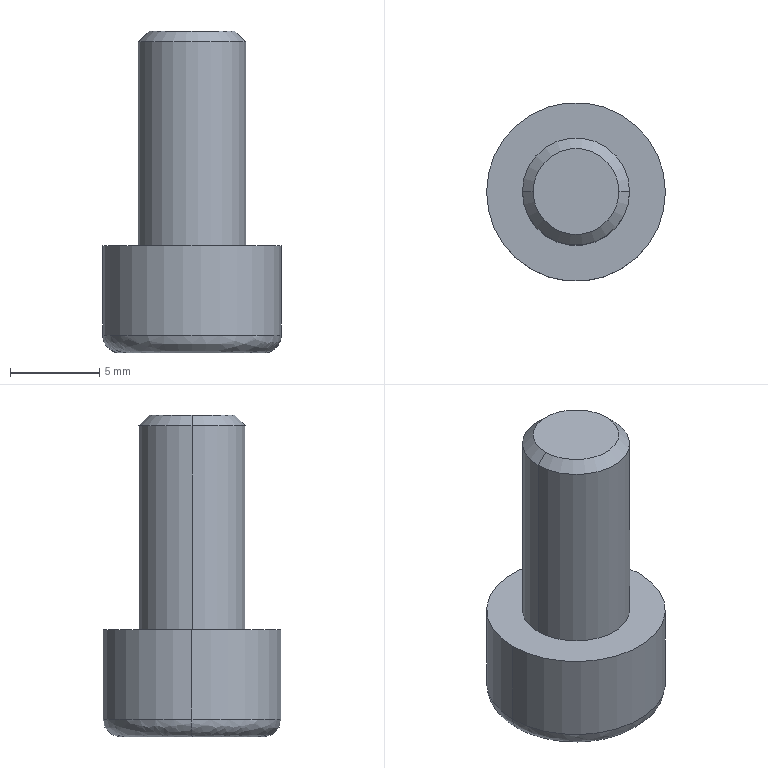Part | STEP file | LE-YZS-M6X12_PN_0002 | 1 solid | 25 faces | box 10 x 10 x 18 mm | volume 726.537 mm3 | plane 15 | cylinder 4 | cone 4 | spline 2 | commonest cylinder face diameters 6 x2 10 x2
STEP:
#1=CARTESIAN_POINT('',(-5.,0.,-5.));
#2=VERTEX_POINT('',#1);
#3=CARTESIAN_POINT('',(5.,0.,-5.));
#4=VERTEX_POINT('',#3);
#5=CARTESIAN_POINT('',(0.,0.,-5.));
#6=DIRECTION('',(0.,0.,1.));
#7=DIRECTION('',(1.,0.,0.));
#8=AXIS2_PLACEMENT_3D('',#5,#6,#7);
#9=CIRCLE('',#8,5.);
#10=EDGE_CURVE('',#2,#4,#9,.T.);
#11=ORIENTED_EDGE('',*,*,#10,.F.);
#12=CARTESIAN_POINT('',(-4.,0.,-6.));
#13=VERTEX_POINT('',#12);
#14=CARTESIAN_POINT('',(-4.,0.,-5.));
#15=DIRECTION('',(0.,-1.,0.));
#16=DIRECTION('',(-1.,0.,0.));
#17=AXIS2_PLACEMENT_3D('',#14,#15,#16);
#18=CIRCLE('',#17,1.);
#19=EDGE_CURVE('',#2,#13,#18,.T.);
#20=ORIENTED_EDGE('',*,*,#19,.T.);
#21=CARTESIAN_POINT('',(4.,0.,-6.));
#22=VERTEX_POINT('',#21);
#23=CARTESIAN_POINT('',(-4.,0.,-6.));
#24=CARTESIAN_POINT('',(-4.,-8.,-6.));
#25=CARTESIAN_POINT('',(4.,-8.,-6.));
#26=CARTESIAN_POINT('',(4.,0.,-6.));
#27=(BOUNDED_CURVE()B_SPLINE_CURVE(3,(#23,#24,#25,#26),.UNSPECIFIED.,.F.,.F.)B_SPLINE_CURVE_WITH_KNOTS((4,4),(0.,1.),.UNSPECIFIED.)CURVE()GEOMETRIC_REPRESENTATION_ITEM()RATIONAL_B_SPLINE_CURVE((1.,0.3333,0.3333,1.))REPRESENTATION_ITEM(''));
#28=EDGE_CURVE('',#13,#22,#27,.T.);
#29=ORIENTED_EDGE('',*,*,#28,.T.);
#30=CARTESIAN_POINT('',(4.,0.,-5.));
#31=DIRECTION('',(0.,1.,0.));
#32=DIRECTION('',(1.,0.,0.));
#33=AXIS2_PLACEMENT_3D('',#30,#31,#32);
#34=CIRCLE('',#33,1.);
#35=EDGE_CURVE('',#4,#22,#34,.T.);
#36=ORIENTED_EDGE('',*,*,#35,.F.);
#37=EDGE_LOOP('',(#11,#20,#29,#36));
#38=FACE_OUTER_BOUND('',#37,.T.);
#39=CARTESIAN_POINT('',(-5.,0.,-5.));
#40=CARTESIAN_POINT('',(-5.,-10.,-5.));
#41=CARTESIAN_POINT('',(5.,-10.,-5.));
#42=CARTESIAN_POINT('',(5.,0.,-5.));
#43=CARTESIAN_POINT('',(-5.,0.,-5.586));
#44=CARTESIAN_POINT('',(-5.,-10.,-5.586));
#45=CARTESIAN_POINT('',(5.,-10.,-5.586));
#46=CARTESIAN_POINT('',(5.,0.,-5.586));
#47=CARTESIAN_POINT('',(-4.586,0.,-6.));
#48=CARTESIAN_POINT('',(-4.586,-9.172,-6.));
#49=CARTESIAN_POINT('',(4.586,-9.172,-6.));
#50=CARTESIAN_POINT('',(4.586,0.,-6.));
#51=CARTESIAN_POINT('',(-4.,0.,-6.));
#52=CARTESIAN_POINT('',(-4.,-8.,-6.));
#53=CARTESIAN_POINT('',(4.,-8.,-6.));
#54=CARTESIAN_POINT('',(4.,0.,-6.));
#55=(BOUNDED_SURFACE()B_SPLINE_SURFACE(3,3,((#39,#40,#41,#42),(#43,#44,#45,#46),(#47,#48,#49,#50),(#51,#52,#53,#54)),.UNSPECIFIED.,.F.,.F.,.F.)B_SPLINE_SURFACE_WITH_KNOTS((4,4),(4,4),(0.,1.),(0.,1.),.UNSPECIFIED.)GEOMETRIC_REPRESENTATION_ITEM()RATIONAL_B_SPLINE_SURFACE(((1.,0.3333,0.3333,1.),(0.8047,0.2682,0.2682,0.8047),(0.8047,0.2682,0.2682,0.8047),(1.,0.3333,0.3333,1.)))REPRESENTATION_ITEM('')SURFACE());
#56=ADVANCED_FACE('',(#38),#55,.T.);
#57=CARTESIAN_POINT('',(-3.,0.,11.4));
#58=VERTEX_POINT('',#57);
#59=CARTESIAN_POINT('',(3.,0.,11.4));
#60=VERTEX_POINT('',#59);
#61=CARTESIAN_POINT('',(0.,0.,11.4));
#62=DIRECTION('',(0.,0.,-1.));
#63=DIRECTION('',(-1.,0.,0.));
#64=AXIS2_PLACEMENT_3D('',#61,#62,#63);
#65=CIRCLE('',#64,3.);
#66=EDGE_CURVE('',#58,#60,#65,.T.);
#67=ORIENTED_EDGE('',*,*,#66,.T.);
#68=CARTESIAN_POINT('',(3.,0.,0.));
#69=VERTEX_POINT('',#68);
#70=CARTESIAN_POINT('',(3.,0.,12.));
#71=DIRECTION('',(0.,0.,-1.));
#72=VECTOR('',#71,1000.);
#73=LINE('',#70,#72);
#74=EDGE_CURVE('',#60,#69,#73,.T.);
#75=ORIENTED_EDGE('',*,*,#74,.T.);
#76=CARTESIAN_POINT('',(-3.,0.,0.));
#77=VERTEX_POINT('',#76);
#78=CARTESIAN_POINT('',(0.,0.,0.));
#79=DIRECTION('',(0.,0.,1.));
#80=DIRECTION('',(-1.,0.,0.));
#81=AXIS2_PLACEMENT_3D('',#78,#79,#80);
#82=CIRCLE('',#81,3.);
#83=EDGE_CURVE('',#69,#77,#82,.T.);
#84=ORIENTED_EDGE('',*,*,#83,.T.);
#85=CARTESIAN_POINT('',(-3.,0.,12.));
#86=DIRECTION('',(0.,0.,-1.));
#87=VECTOR('',#86,1000.);
#88=LINE('',#85,#87);
#89=EDGE_CURVE('',#58,#77,#88,.T.);
#90=ORIENTED_EDGE('',*,*,#89,.F.);
#91=EDGE_LOOP('',(#67,#75,#84,#90));
#92=FACE_OUTER_BOUND('',#91,.T.);
#93=CARTESIAN_POINT('',(0.,0.,12.));
#94=DIRECTION('',(0.,0.,-1.));
#95=DIRECTION('',(-1.,0.,0.));
#96=AXIS2_PLACEMENT_3D('',#93,#94,#95);
#97=CYLINDRICAL_SURFACE('',#96,3.);
#98=ADVANCED_FACE('',(#92),#97,.T.);
#99=CARTESIAN_POINT('',(-2.4,0.,12.));
#100=VERTEX_POINT('',#99);
#101=CARTESIAN_POINT('',(2.4,0.,12.));
#102=VERTEX_POINT('',#101);
#103=CARTESIAN_POINT('',(0.,0.,12.));
#104=DIRECTION('',(0.,0.,-1.));
#105=DIRECTION('',(-1.,0.,0.));
#106=AXIS2_PLACEMENT_3D('',#103,#104,#105);
#107=CIRCLE('',#106,2.4);
#108=EDGE_CURVE('',#100,#102,#107,.T.);
#109=ORIENTED_EDGE('',*,*,#108,.T.);
#110=CARTESIAN_POINT('',(3.,0.,11.4));
#111=DIRECTION('',(0.7071,0.,-0.7071));
#112=VECTOR('',#111,1000.);
#113=LINE('',#110,#112);
#114=EDGE_CURVE('',#102,#60,#113,.T.);
#115=ORIENTED_EDGE('',*,*,#114,.T.);
#116=ORIENTED_EDGE('',*,*,#66,.F.);
#117=CARTESIAN_POINT('',(-3.,0.,11.4));
#118=DIRECTION('',(-0.7071,0.,-0.7071));
#119=VECTOR('',#118,1000.);
#120=LINE('',#117,#119);
#121=EDGE_CURVE('',#100,#58,#120,.T.);
#122=ORIENTED_EDGE('',*,*,#121,.F.);
#123=EDGE_LOOP('',(#109,#115,#116,#122));
#124=FACE_OUTER_BOUND('',#123,.T.);
#125=CARTESIAN_POINT('',(0.,0.,11.4));
#126=DIRECTION('',(0.,0.,-1.));
#127=DIRECTION('',(-1.,0.,0.));
#128=AXIS2_PLACEMENT_3D('',#125,#126,#127);
#129=CONICAL_SURFACE('',#128,3.,0.7854);
#130=ADVANCED_FACE('',(#124),#129,.T.);
#131=CARTESIAN_POINT('',(0.,0.,-5.));
#132=DIRECTION('',(0.,0.,1.));
#133=DIRECTION('',(1.,0.,0.));
#134=AXIS2_PLACEMENT_3D('',#131,#132,#133);
#135=CIRCLE('',#134,5.);
#136=EDGE_CURVE('',#4,#2,#135,.T.);
#137=ORIENTED_EDGE('',*,*,#136,.T.);
#138=CARTESIAN_POINT('',(-5.,0.,0.));
#139=VERTEX_POINT('',#138);
#140=CARTESIAN_POINT('',(-5.,0.,-6.));
#141=DIRECTION('',(0.,0.,1.));
#142=VECTOR('',#141,1000.);
#143=LINE('',#140,#142);
#144=EDGE_CURVE('',#2,#139,#143,.T.);
#145=ORIENTED_EDGE('',*,*,#144,.T.);
#146=CARTESIAN_POINT('',(5.,0.,0.));
#147=VERTEX_POINT('',#146);
#148=CARTESIAN_POINT('',(0.,0.,0.));
#149=DIRECTION('',(0.,0.,1.));
#150=DIRECTION('',(1.,0.,0.));
#151=AXIS2_PLACEMENT_3D('',#148,#149,#150);
#152=CIRCLE('',#151,5.);
#153=EDGE_CURVE('',#147,#139,#152,.T.);
#154=ORIENTED_EDGE('',*,*,#153,.F.);
#155=CARTESIAN_POINT('',(5.,0.,-6.));
#156=DIRECTION('',(0.,0.,1.));
#157=VECTOR('',#156,1000.);
#158=LINE('',#155,#157);
#159=EDGE_CURVE('',#4,#147,#158,.T.);
#160=ORIENTED_EDGE('',*,*,#159,.F.);
#161=EDGE_LOOP('',(#137,#145,#154,#160));
#162=FACE_OUTER_BOUND('',#161,.T.);
#163=CARTESIAN_POINT('',(0.,0.,-6.));
#164=DIRECTION('',(0.,0.,1.));
#165=DIRECTION('',(1.,0.,0.));
#166=AXIS2_PLACEMENT_3D('',#163,#164,#165);
#167=CYLINDRICAL_SURFACE('',#166,5.);
#168=ADVANCED_FACE('',(#162),#167,.T.);
#169=CARTESIAN_POINT('',(0.,0.,-1.557));
#170=VERTEX_POINT('',#169);
#171=CARTESIAN_POINT('',(-2.5,0.,-3.));
#172=VERTEX_POINT('',#171);
#173=CARTESIAN_POINT('',(-2.5,0.,-3.));
#174=DIRECTION('',(-0.866,0.,-0.5));
#175=VECTOR('',#174,1000.);
#176=LINE('',#173,#175);
#177=EDGE_CURVE('',#170,#172,#176,.T.);
#178=ORIENTED_EDGE('',*,*,#177,.F.);
#179=CARTESIAN_POINT('',(2.5,0.,-3.));
#180=VERTEX_POINT('',#179);
#181=CARTESIAN_POINT('',(2.5,0.,-3.));
#182=DIRECTION('',(0.866,0.,-0.5));
#183=VECTOR('',#182,1000.);
#184=LINE('',#181,#183);
#185=EDGE_CURVE('',#170,#180,#184,.T.);
#186=ORIENTED_EDGE('',*,*,#185,.T.);
#187=CARTESIAN_POINT('',(2.165,-1.25,-3.));
#188=VERTEX_POINT('',#187);
#189=CARTESIAN_POINT('',(0.,0.,-3.));
#190=DIRECTION('',(0.,0.,1.));
#191=DIRECTION('',(-1.,0.,0.));
#192=AXIS2_PLACEMENT_3D('',#189,#190,#191);
#193=CIRCLE('',#192,2.5);
#194=EDGE_CURVE('',#188,#180,#193,.T.);
#195=ORIENTED_EDGE('',*,*,#194,.F.);
#196=CARTESIAN_POINT('',(0.,-2.5,-3.));
#197=VERTEX_POINT('',#196);
#198=CARTESIAN_POINT('',(0.,0.,-3.));
#199=DIRECTION('',(0.,0.,-1.));
#200=DIRECTION('',(-1.,0.,0.));
#201=AXIS2_PLACEMENT_3D('',#198,#199,#200);
#202=CIRCLE('',#201,2.5);
#203=EDGE_CURVE('',#188,#197,#202,.T.);
#204=ORIENTED_EDGE('',*,*,#203,.T.);
#205=CARTESIAN_POINT('',(-2.165,-1.25,-3.));
#206=VERTEX_POINT('',#205);
#207=CARTESIAN_POINT('',(0.,0.,-3.));
#208=DIRECTION('',(0.,0.,1.));
#209=DIRECTION('',(-1.,0.,0.));
#210=AXIS2_PLACEMENT_3D('',#207,#208,#209);
#211=CIRCLE('',#210,2.5);
#212=EDGE_CURVE('',#206,#197,#211,.T.);
#213=ORIENTED_EDGE('',*,*,#212,.F.);
#214=CARTESIAN_POINT('',(0.,0.,-3.));
#215=DIRECTION('',(0.,0.,1.));
#216=DIRECTION('',(-1.,0.,0.));
#217=AXIS2_PLACEMENT_3D('',#214,#215,#216);
#218=CIRCLE('',#217,2.5);
#219=EDGE_CURVE('',#172,#206,#218,.T.);
#220=ORIENTED_EDGE('',*,*,#219,.F.);
#221=EDGE_LOOP('',(#178,#186,#195,#204,#213,#220));
#222=FACE_OUTER_BOUND('',#221,.T.);
#223=CARTESIAN_POINT('',(0.,0.,-3.));
#224=DIRECTION('',(0.,0.,-1.));
#225=DIRECTION('',(-1.,0.,0.));
#226=AXIS2_PLACEMENT_3D('',#223,#224,#225);
#227=CONICAL_SURFACE('',#226,2.5,1.047);
#228=ADVANCED_FACE('',(#222),#227,.F.);
#229=ORIENTED_EDGE('',*,*,#74,.F.);
#230=CARTESIAN_POINT('',(0.,0.,11.4));
#231=DIRECTION('',(0.,0.,-1.));
#232=DIRECTION('',(-1.,0.,0.));
#233=AXIS2_PLACEMENT_3D('',#230,#231,#232);
#234=CIRCLE('',#233,3.);
#235=EDGE_CURVE('',#60,#58,#234,.T.);
#236=ORIENTED_EDGE('',*,*,#235,.T.);
#237=ORIENTED_EDGE('',*,*,#89,.T.);
#238=CARTESIAN_POINT('',(0.,0.,0.));
#239=DIRECTION('',(0.,0.,1.));
#240=DIRECTION('',(-1.,0.,0.));
#241=AXIS2_PLACEMENT_3D('',#238,#239,#240);
#242=CIRCLE('',#241,3.);
#243=EDGE_CURVE('',#77,#69,#242,.T.);
#244=ORIENTED_EDGE('',*,*,#243,.T.);
#245=EDGE_LOOP('',(#229,#236,#237,#244));
#246=FACE_OUTER_BOUND('',#245,.T.);
#247=CARTESIAN_POINT('',(0.,0.,12.));
#248=DIRECTION('',(0.,0.,-1.));
#249=DIRECTION('',(-1.,0.,0.));
#250=AXIS2_PLACEMENT_3D('',#247,#248,#249);
#251=CYLINDRICAL_SURFACE('',#250,3.);
#252=ADVANCED_FACE('',(#246),#251,.T.);
#253=ORIENTED_EDGE('',*,*,#153,.T.);
#254=CARTESIAN_POINT('',(0.,0.,0.));
#255=DIRECTION('',(0.,0.,1.));
#256=DIRECTION('',(1.,0.,0.));
#257=AXIS2_PLACEMENT_3D('',#254,#255,#256);
#258=CIRCLE('',#257,5.);
#259=EDGE_CURVE('',#139,#147,#258,.T.);
#260=ORIENTED_EDGE('',*,*,#259,.T.);
#261=EDGE_LOOP('',(#253,#260));
#262=FACE_OUTER_BOUND('',#261,.T.);
#263=ORIENTED_EDGE('',*,*,#243,.F.);
#264=ORIENTED_EDGE('',*,*,#83,.F.);
#265=EDGE_LOOP('',(#263,#264));
#266=FACE_BOUND('',#265,.T.);
#267=CARTESIAN_POINT('',(0.,0.,0.));
#268=DIRECTION('',(0.,0.,1.));
#269=DIRECTION('',(1.,0.,0.));
#270=AXIS2_PLACEMENT_3D('',#267,#268,#269);
#271=PLANE('',#270);
#272=ADVANCED_FACE('',(#262,#266),#271,.T.);
#273=ORIENTED_EDGE('',*,*,#114,.F.);
#274=CARTESIAN_POINT('',(0.,0.,12.));
#275=DIRECTION('',(0.,0.,-1.));
#276=DIRECTION('',(-1.,0.,0.));
#277=AXIS2_PLACEMENT_3D('',#274,#275,#276);
#278=CIRCLE('',#277,2.4);
#279=EDGE_CURVE('',#102,#100,#278,.T.);
#280=ORIENTED_EDGE('',*,*,#279,.T.);
#281=ORIENTED_EDGE('',*,*,#121,.T.);
#282=ORIENTED_EDGE('',*,*,#235,.F.);
#283=EDGE_LOOP('',(#273,#280,#281,#282));
#284=FACE_OUTER_BOUND('',#283,.T.);
#285=CARTESIAN_POINT('',(0.,0.,11.4));
#286=DIRECTION('',(0.,0.,-1.));
#287=DIRECTION('',(-1.,0.,0.));
#288=AXIS2_PLACEMENT_3D('',#285,#286,#287);
#289=CONICAL_SURFACE('',#288,3.,0.7854);
#290=ADVANCED_FACE('',(#284),#289,.T.);
#291=ORIENTED_EDGE('',*,*,#144,.F.);
#292=ORIENTED_EDGE('',*,*,#10,.T.);
#293=ORIENTED_EDGE('',*,*,#159,.T.);
#294=ORIENTED_EDGE('',*,*,#259,.F.);
#295=EDGE_LOOP('',(#291,#292,#293,#294));
#296=FACE_OUTER_BOUND('',#295,.T.);
#297=CARTESIAN_POINT('',(0.,0.,-6.));
#298=DIRECTION('',(0.,0.,1.));
#299=DIRECTION('',(1.,0.,0.));
#300=AXIS2_PLACEMENT_3D('',#297,#298,#299);
#301=CYLINDRICAL_SURFACE('',#300,5.);
#302=ADVANCED_FACE('',(#296),#301,.T.);
#303=ORIENTED_EDGE('',*,*,#108,.F.);
#304=ORIENTED_EDGE('',*,*,#279,.F.);
#305=EDGE_LOOP('',(#303,#304));
#306=FACE_OUTER_BOUND('',#305,.T.);
#307=CARTESIAN_POINT('',(0.,0.,12.));
#308=DIRECTION('',(0.,0.,-1.));
#309=DIRECTION('',(-1.,0.,0.));
#310=AXIS2_PLACEMENT_3D('',#307,#308,#309);
#311=PLANE('',#310);
#312=ADVANCED_FACE('',(#306),#311,.F.);
#313=ORIENTED_EDGE('',*,*,#19,.F.);
#314=ORIENTED_EDGE('',*,*,#136,.F.);
#315=ORIENTED_EDGE('',*,*,#35,.T.);
#316=CARTESIAN_POINT('',(4.,0.,-6.));
#317=CARTESIAN_POINT('',(4.,8.,-6.));
#318=CARTESIAN_POINT('',(-4.,8.,-6.));
#319=CARTESIAN_POINT('',(-4.,0.,-6.));
#320=(BOUNDED_CURVE()B_SPLINE_CURVE(3,(#316,#317,#318,#319),.UNSPECIFIED.,.F.,.F.)B_SPLINE_CURVE_WITH_KNOTS((4,4),(0.,1.),.UNSPECIFIED.)CURVE()GEOMETRIC_REPRESENTATION_ITEM()RATIONAL_B_SPLINE_CURVE((1.,0.3333,0.3333,1.))REPRESENTATION_ITEM(''));
#321=EDGE_CURVE('',#22,#13,#320,.T.);
#322=ORIENTED_EDGE('',*,*,#321,.T.);
#323=EDGE_LOOP('',(#313,#314,#315,#322));
#324=FACE_OUTER_BOUND('',#323,.T.);
#325=CARTESIAN_POINT('',(5.,0.,-5.));
#326=CARTESIAN_POINT('',(5.,10.,-5.));
#327=CARTESIAN_POINT('',(-5.,10.,-5.));
#328=CARTESIAN_POINT('',(-5.,0.,-5.));
#329=CARTESIAN_POINT('',(5.,0.,-5.586));
#330=CARTESIAN_POINT('',(5.,10.,-5.586));
#331=CARTESIAN_POINT('',(-5.,10.,-5.586));
#332=CARTESIAN_POINT('',(-5.,0.,-5.586));
#333=CARTESIAN_POINT('',(4.586,0.,-6.));
#334=CARTESIAN_POINT('',(4.586,9.172,-6.));
#335=CARTESIAN_POINT('',(-4.586,9.172,-6.));
#336=CARTESIAN_POINT('',(-4.586,0.,-6.));
#337=CARTESIAN_POINT('',(4.,0.,-6.));
#338=CARTESIAN_POINT('',(4.,8.,-6.));
#339=CARTESIAN_POINT('',(-4.,8.,-6.));
#340=CARTESIAN_POINT('',(-4.,0.,-6.));
#341=(BOUNDED_SURFACE()B_SPLINE_SURFACE(3,3,((#325,#326,#327,#328),(#329,#330,#331,#332),(#333,#334,#335,#336),(#337,#338,#339,#340)),.UNSPECIFIED.,.F.,.F.,.T.)B_SPLINE_SURFACE_WITH_KNOTS((4,4),(4,4),(0.,1.),(0.,1.),.UNSPECIFIED.)GEOMETRIC_REPRESENTATION_ITEM()RATIONAL_B_SPLINE_SURFACE(((1.,0.3333,0.3333,1.),(0.8047,0.2682,0.2682,0.8047),(0.8047,0.2682,0.2682,0.8047),(1.,0.3333,0.3333,1.)))REPRESENTATION_ITEM('')SURFACE());
#342=ADVANCED_FACE('',(#324),#341,.T.);
#343=CARTESIAN_POINT('',(-1.443,2.5,-6.));
#344=VERTEX_POINT('',#343);
#345=CARTESIAN_POINT('',(1.443,2.5,-6.));
#346=VERTEX_POINT('',#345);
#347=CARTESIAN_POINT('',(0.,2.5,-6.));
#348=DIRECTION('',(1.,0.,0.));
#349=VECTOR('',#348,1000.);
#350=LINE('',#347,#349);
#351=EDGE_CURVE('',#344,#346,#350,.T.);
#352=ORIENTED_EDGE('',*,*,#351,.F.);
#353=CARTESIAN_POINT('',(-2.887,0.,-6.));
#354=VERTEX_POINT('',#353);
#355=CARTESIAN_POINT('',(-2.887,0.,-6.));
#356=DIRECTION('',(0.5,0.866,0.));
#357=VECTOR('',#356,1000.);
#358=LINE('',#355,#357);
#359=EDGE_CURVE('',#354,#344,#358,.T.);
#360=ORIENTED_EDGE('',*,*,#359,.F.);
#361=CARTESIAN_POINT('',(-1.443,-2.5,-6.));
#362=VERTEX_POINT('',#361);
#363=CARTESIAN_POINT('',(-1.443,-2.5,-6.));
#364=DIRECTION('',(-0.5,0.866,0.));
#365=VECTOR('',#364,1000.);
#366=LINE('',#363,#365);
#367=EDGE_CURVE('',#362,#354,#366,.T.);
#368=ORIENTED_EDGE('',*,*,#367,.F.);
#369=CARTESIAN_POINT('',(1.443,-2.5,-6.));
#370=VERTEX_POINT('',#369);
#371=CARTESIAN_POINT('',(0.,-2.5,-6.));
#372=DIRECTION('',(-1.,0.,0.));
#373=VECTOR('',#372,1000.);
#374=LINE('',#371,#373);
#375=EDGE_CURVE('',#370,#362,#374,.T.);
#376=ORIENTED_EDGE('',*,*,#375,.F.);
#377=CARTESIAN_POINT('',(2.887,0.,-6.));
#378=VERTEX_POINT('',#377);
#379=CARTESIAN_POINT('',(2.887,0.,-6.));
#380=DIRECTION('',(-0.5,-0.866,0.));
#381=VECTOR('',#380,1000.);
#382=LINE('',#379,#381);
#383=EDGE_CURVE('',#378,#370,#382,.T.);
#384=ORIENTED_EDGE('',*,*,#383,.F.);
#385=CARTESIAN_POINT('',(1.443,2.5,-6.));
#386=DIRECTION('',(0.5,-0.866,0.));
#387=VECTOR('',#386,1000.);
#388=LINE('',#385,#387);
#389=EDGE_CURVE('',#346,#378,#388,.T.);
#390=ORIENTED_EDGE('',*,*,#389,.F.);
#391=EDGE_LOOP('',(#352,#360,#368,#376,#384,#390));
#392=FACE_BOUND('',#391,.T.);
#393=ORIENTED_EDGE('',*,*,#321,.F.);
#394=ORIENTED_EDGE('',*,*,#28,.F.);
#395=EDGE_LOOP('',(#393,#394));
#396=FACE_OUTER_BOUND('',#395,.T.);
#397=CARTESIAN_POINT('',(0.,0.,-6.));
#398=DIRECTION('',(0.,0.,1.));
#399=DIRECTION('',(1.,0.,0.));
#400=AXIS2_PLACEMENT_3D('',#397,#398,#399);
#401=PLANE('',#400);
#402=ADVANCED_FACE('',(#392,#396),#401,.F.);
#403=CARTESIAN_POINT('',(2.165,1.25,-3.));
#404=VERTEX_POINT('',#403);
#405=CARTESIAN_POINT('',(1.443,2.5,-3.));
#406=VERTEX_POINT('',#405);
#407=CARTESIAN_POINT('',(2.165,1.25,-3.));
#408=DIRECTION('',(-0.5,0.866,0.));
#409=VECTOR('',#408,1000.);
#410=LINE('',#407,#409);
#411=EDGE_CURVE('',#404,#406,#410,.T.);
#412=ORIENTED_EDGE('',*,*,#411,.T.);
#413=CARTESIAN_POINT('',(1.443,2.5,-3.));
#414=DIRECTION('',(0.,0.,-1.));
#415=VECTOR('',#414,1000.);
#416=LINE('',#413,#415);
#417=EDGE_CURVE('',#406,#346,#416,.T.);
#418=ORIENTED_EDGE('',*,*,#417,.T.);
#419=ORIENTED_EDGE('',*,*,#389,.T.);
#420=CARTESIAN_POINT('',(2.887,0.,-3.));
#421=VERTEX_POINT('',#420);
#422=CARTESIAN_POINT('',(2.887,0.,-3.));
#423=DIRECTION('',(0.,0.,1.));
#424=VECTOR('',#423,1000.);
#425=LINE('',#422,#424);
#426=EDGE_CURVE('',#378,#421,#425,.T.);
#427=ORIENTED_EDGE('',*,*,#426,.T.);
#428=CARTESIAN_POINT('',(2.887,0.,-3.));
#429=DIRECTION('',(-0.5,0.866,0.));
#430=VECTOR('',#429,1000.);
#431=LINE('',#428,#430);
#432=EDGE_CURVE('',#421,#404,#431,.T.);
#433=ORIENTED_EDGE('',*,*,#432,.T.);
#434=EDGE_LOOP('',(#412,#418,#419,#427,#433));
#435=FACE_OUTER_BOUND('',#434,.T.);
#436=CARTESIAN_POINT('',(2.887,0.,-3.));
#437=DIRECTION('',(-0.866,-0.5,0.));
#438=DIRECTION('',(0.5,-0.866,0.));
#439=AXIS2_PLACEMENT_3D('',#436,#437,#438);
#440=PLANE('',#439);
#441=ADVANCED_FACE('',(#435),#440,.T.);
#442=CARTESIAN_POINT('',(0.,2.5,-3.));
#443=VERTEX_POINT('',#442);
#444=CARTESIAN_POINT('',(-1.443,2.5,-3.));
#445=VERTEX_POINT('',#444);
#446=CARTESIAN_POINT('',(0.,2.5,-3.));
#447=DIRECTION('',(-1.,0.,0.));
#448=VECTOR('',#447,1000.);
#449=LINE('',#446,#448);
#450=EDGE_CURVE('',#443,#445,#449,.T.);
#451=ORIENTED_EDGE('',*,*,#450,.T.);
#452=CARTESIAN_POINT('',(-1.443,2.5,-3.));
#453=DIRECTION('',(0.,0.,-1.));
#454=VECTOR('',#453,1000.);
#455=LINE('',#452,#454);
#456=EDGE_CURVE('',#445,#344,#455,.T.);
#457=ORIENTED_EDGE('',*,*,#456,.T.);
#458=ORIENTED_EDGE('',*,*,#351,.T.);
#459=ORIENTED_EDGE('',*,*,#417,.F.);
#460=CARTESIAN_POINT('',(0.,2.5,-3.));
#461=DIRECTION('',(-1.,0.,0.));
#462=VECTOR('',#461,1000.);
#463=LINE('',#460,#462);
#464=EDGE_CURVE('',#406,#443,#463,.T.);
#465=ORIENTED_EDGE('',*,*,#464,.T.);
#466=EDGE_LOOP('',(#451,#457,#458,#459,#465));
#467=FACE_OUTER_BOUND('',#466,.T.);
#468=CARTESIAN_POINT('',(1.443,2.5,-3.));
#469=DIRECTION('',(0.,-1.,0.));
#470=DIRECTION('',(0.,0.,-1.));
#471=AXIS2_PLACEMENT_3D('',#468,#469,#470);
#472=PLANE('',#471);
#473=ADVANCED_FACE('',(#467),#472,.T.);
#474=CARTESIAN_POINT('',(-2.165,1.25,-3.));
#475=VERTEX_POINT('',#474);
#476=CARTESIAN_POINT('',(-2.887,0.,-3.));
#477=VERTEX_POINT('',#476);
#478=CARTESIAN_POINT('',(-1.443,2.5,-3.));
#479=DIRECTION('',(-0.5,-0.866,0.));
#480=VECTOR('',#479,1000.);
#481=LINE('',#478,#480);
#482=EDGE_CURVE('',#475,#477,#481,.T.);
#483=ORIENTED_EDGE('',*,*,#482,.T.);
#484=CARTESIAN_POINT('',(-2.887,0.,-3.));
#485=DIRECTION('',(0.,0.,-1.));
#486=VECTOR('',#485,1000.);
#487=LINE('',#484,#486);
#488=EDGE_CURVE('',#477,#354,#487,.T.);
#489=ORIENTED_EDGE('',*,*,#488,.T.);
#490=ORIENTED_EDGE('',*,*,#359,.T.);
#491=ORIENTED_EDGE('',*,*,#456,.F.);
#492=CARTESIAN_POINT('',(-1.443,2.5,-3.));
#493=DIRECTION('',(-0.5,-0.866,0.));
#494=VECTOR('',#493,1000.);
#495=LINE('',#492,#494);
#496=EDGE_CURVE('',#445,#475,#495,.T.);
#497=ORIENTED_EDGE('',*,*,#496,.T.);
#498=EDGE_LOOP('',(#483,#489,#490,#491,#497));
#499=FACE_OUTER_BOUND('',#498,.T.);
#500=CARTESIAN_POINT('',(-1.443,2.5,-3.));
#501=DIRECTION('',(0.866,-0.5,0.));
#502=DIRECTION('',(0.5,0.866,0.));
#503=AXIS2_PLACEMENT_3D('',#500,#501,#502);
#504=PLANE('',#503);
#505=ADVANCED_FACE('',(#499),#504,.T.);
#506=CARTESIAN_POINT('',(-1.443,-2.5,-3.));
#507=VERTEX_POINT('',#506);
#508=CARTESIAN_POINT('',(-2.165,-1.25,-3.));
#509=DIRECTION('',(0.5,-0.866,0.));
#510=VECTOR('',#509,1000.);
#511=LINE('',#508,#510);
#512=EDGE_CURVE('',#206,#507,#511,.T.);
#513=ORIENTED_EDGE('',*,*,#512,.T.);
#514=CARTESIAN_POINT('',(-1.443,-2.5,-3.));
#515=DIRECTION('',(0.,0.,-1.));
#516=VECTOR('',#515,1000.);
#517=LINE('',#514,#516);
#518=EDGE_CURVE('',#507,#362,#517,.T.);
#519=ORIENTED_EDGE('',*,*,#518,.T.);
#520=ORIENTED_EDGE('',*,*,#367,.T.);
#521=ORIENTED_EDGE('',*,*,#488,.F.);
#522=CARTESIAN_POINT('',(-2.887,0.,-3.));
#523=DIRECTION('',(0.5,-0.866,0.));
#524=VECTOR('',#523,1000.);
#525=LINE('',#522,#524);
#526=EDGE_CURVE('',#477,#206,#525,.T.);
#527=ORIENTED_EDGE('',*,*,#526,.T.);
#528=EDGE_LOOP('',(#513,#519,#520,#521,#527));
#529=FACE_OUTER_BOUND('',#528,.T.);
#530=CARTESIAN_POINT('',(-2.887,0.,-3.));
#531=DIRECTION('',(0.866,0.5,0.));
#532=DIRECTION('',(-0.5,0.866,0.));
#533=AXIS2_PLACEMENT_3D('',#530,#531,#532);
#534=PLANE('',#533);
#535=ADVANCED_FACE('',(#529),#534,.T.);
#536=CARTESIAN_POINT('',(1.443,-2.5,-3.));
#537=VERTEX_POINT('',#536);
#538=CARTESIAN_POINT('',(-1.443,-2.5,-3.));
#539=DIRECTION('',(1.,0.,0.));
#540=VECTOR('',#539,1000.);
#541=LINE('',#538,#540);
#542=EDGE_CURVE('',#197,#537,#541,.T.);
#543=ORIENTED_EDGE('',*,*,#542,.T.);
#544=CARTESIAN_POINT('',(1.443,-2.5,-3.));
#545=DIRECTION('',(0.,0.,-1.));
#546=VECTOR('',#545,1000.);
#547=LINE('',#544,#546);
#548=EDGE_CURVE('',#537,#370,#547,.T.);
#549=ORIENTED_EDGE('',*,*,#548,.T.);
#550=ORIENTED_EDGE('',*,*,#375,.T.);
#551=ORIENTED_EDGE('',*,*,#518,.F.);
#552=CARTESIAN_POINT('',(0.,-2.5,-3.));
#553=DIRECTION('',(1.,0.,0.));
#554=VECTOR('',#553,1000.);
#555=LINE('',#552,#554);
#556=EDGE_CURVE('',#507,#197,#555,.T.);
#557=ORIENTED_EDGE('',*,*,#556,.T.);
#558=EDGE_LOOP('',(#543,#549,#550,#551,#557));
#559=FACE_OUTER_BOUND('',#558,.T.);
#560=CARTESIAN_POINT('',(-1.443,-2.5,-3.));
#561=DIRECTION('',(0.,1.,0.));
#562=DIRECTION('',(-1.,0.,0.));
#563=AXIS2_PLACEMENT_3D('',#560,#561,#562);
#564=PLANE('',#563);
#565=ADVANCED_FACE('',(#559),#564,.T.);
#566=CARTESIAN_POINT('',(1.443,-2.5,-3.));
#567=DIRECTION('',(0.5,0.866,0.));
#568=VECTOR('',#567,1000.);
#569=LINE('',#566,#568);
#570=EDGE_CURVE('',#188,#421,#569,.T.);
#571=ORIENTED_EDGE('',*,*,#570,.T.);
#572=ORIENTED_EDGE('',*,*,#426,.F.);
#573=ORIENTED_EDGE('',*,*,#383,.T.);
#574=ORIENTED_EDGE('',*,*,#548,.F.);
#575=CARTESIAN_POINT('',(1.443,-2.5,-3.));
#576=DIRECTION('',(0.5,0.866,0.));
#577=VECTOR('',#576,1000.);
#578=LINE('',#575,#577);
#579=EDGE_CURVE('',#537,#188,#578,.T.);
#580=ORIENTED_EDGE('',*,*,#579,.T.);
#581=EDGE_LOOP('',(#571,#572,#573,#574,#580));
#582=FACE_OUTER_BOUND('',#581,.T.);
#583=CARTESIAN_POINT('',(1.443,-2.5,-3.));
#584=DIRECTION('',(-0.866,0.5,0.));
#585=DIRECTION('',(-0.5,-0.866,0.));
#586=AXIS2_PLACEMENT_3D('',#583,#584,#585);
#587=PLANE('',#586);
#588=ADVANCED_FACE('',(#582),#587,.T.);
#589=ORIENTED_EDGE('',*,*,#194,.T.);
#590=CARTESIAN_POINT('',(0.,0.,-3.));
#591=DIRECTION('',(0.,0.,1.));
#592=DIRECTION('',(-1.,0.,0.));
#593=AXIS2_PLACEMENT_3D('',#590,#591,#592);
#594=CIRCLE('',#593,2.5);
#595=EDGE_CURVE('',#180,#404,#594,.T.);
#596=ORIENTED_EDGE('',*,*,#595,.T.);
#597=ORIENTED_EDGE('',*,*,#432,.F.);
#598=ORIENTED_EDGE('',*,*,#570,.F.);
#599=EDGE_LOOP('',(#589,#596,#597,#598));
#600=FACE_OUTER_BOUND('',#599,.T.);
#601=CARTESIAN_POINT('',(0.,0.,-3.));
#602=DIRECTION('',(0.,0.,1.));
#603=DIRECTION('',(1.,0.,0.));
#604=AXIS2_PLACEMENT_3D('',#601,#602,#603);
#605=PLANE('',#604);
#606=ADVANCED_FACE('',(#600),#605,.F.);
#607=ORIENTED_EDGE('',*,*,#482,.F.);
#608=CARTESIAN_POINT('',(0.,0.,-3.));
#609=DIRECTION('',(0.,0.,1.));
#610=DIRECTION('',(-1.,0.,0.));
#611=AXIS2_PLACEMENT_3D('',#608,#609,#610);
#612=CIRCLE('',#611,2.5);
#613=EDGE_CURVE('',#475,#172,#612,.T.);
#614=ORIENTED_EDGE('',*,*,#613,.T.);
#615=ORIENTED_EDGE('',*,*,#219,.T.);
#616=ORIENTED_EDGE('',*,*,#526,.F.);
#617=EDGE_LOOP('',(#607,#614,#615,#616));
#618=FACE_OUTER_BOUND('',#617,.T.);
#619=CARTESIAN_POINT('',(0.,0.,-3.));
#620=DIRECTION('',(0.,0.,1.));
#621=DIRECTION('',(1.,0.,0.));
#622=AXIS2_PLACEMENT_3D('',#619,#620,#621);
#623=PLANE('',#622);
#624=ADVANCED_FACE('',(#618),#623,.F.);
#625=ORIENTED_EDGE('',*,*,#203,.F.);
#626=ORIENTED_EDGE('',*,*,#579,.F.);
#627=ORIENTED_EDGE('',*,*,#542,.F.);
#628=EDGE_LOOP('',(#625,#626,#627));
#629=FACE_OUTER_BOUND('',#628,.T.);
#630=CARTESIAN_POINT('',(0.,0.,-3.));
#631=DIRECTION('',(0.,0.,1.));
#632=DIRECTION('',(1.,0.,0.));
#633=AXIS2_PLACEMENT_3D('',#630,#631,#632);
#634=PLANE('',#633);
#635=ADVANCED_FACE('',(#629),#634,.F.);
#636=ORIENTED_EDGE('',*,*,#185,.F.);
#637=ORIENTED_EDGE('',*,*,#177,.T.);
#638=ORIENTED_EDGE('',*,*,#613,.F.);
#639=CARTESIAN_POINT('',(0.,0.,-3.));
#640=DIRECTION('',(0.,0.,1.));
#641=DIRECTION('',(-1.,0.,0.));
#642=AXIS2_PLACEMENT_3D('',#639,#640,#641);
#643=CIRCLE('',#642,2.5);
#644=EDGE_CURVE('',#443,#475,#643,.T.);
#645=ORIENTED_EDGE('',*,*,#644,.F.);
#646=CARTESIAN_POINT('',(0.,0.,-3.));
#647=DIRECTION('',(0.,0.,1.));
#648=DIRECTION('',(-1.,0.,0.));
#649=AXIS2_PLACEMENT_3D('',#646,#647,#648);
#650=CIRCLE('',#649,2.5);
#651=EDGE_CURVE('',#404,#443,#650,.T.);
#652=ORIENTED_EDGE('',*,*,#651,.F.);
#653=ORIENTED_EDGE('',*,*,#595,.F.);
#654=EDGE_LOOP('',(#636,#637,#638,#645,#652,#653));
#655=FACE_OUTER_BOUND('',#654,.T.);
#656=CARTESIAN_POINT('',(0.,0.,-3.));
#657=DIRECTION('',(0.,0.,-1.));
#658=DIRECTION('',(-1.,0.,0.));
#659=AXIS2_PLACEMENT_3D('',#656,#657,#658);
#660=CONICAL_SURFACE('',#659,2.5,1.047);
#661=ADVANCED_FACE('',(#655),#660,.F.);
#662=ORIENTED_EDGE('',*,*,#212,.T.);
#663=ORIENTED_EDGE('',*,*,#556,.F.);
#664=ORIENTED_EDGE('',*,*,#512,.F.);
#665=EDGE_LOOP('',(#662,#663,#664));
#666=FACE_OUTER_BOUND('',#665,.T.);
#667=CARTESIAN_POINT('',(0.,0.,-3.));
#668=DIRECTION('',(0.,0.,1.));
#669=DIRECTION('',(1.,0.,0.));
#670=AXIS2_PLACEMENT_3D('',#667,#668,#669);
#671=PLANE('',#670);
#672=ADVANCED_FACE('',(#666),#671,.F.);
#673=ORIENTED_EDGE('',*,*,#644,.T.);
#674=ORIENTED_EDGE('',*,*,#496,.F.);
#675=ORIENTED_EDGE('',*,*,#450,.F.);
#676=EDGE_LOOP('',(#673,#674,#675));
#677=FACE_OUTER_BOUND('',#676,.T.);
#678=CARTESIAN_POINT('',(0.,0.,-3.));
#679=DIRECTION('',(0.,0.,1.));
#680=DIRECTION('',(1.,0.,0.));
#681=AXIS2_PLACEMENT_3D('',#678,#679,#680);
#682=PLANE('',#681);
#683=ADVANCED_FACE('',(#677),#682,.F.);
#684=ORIENTED_EDGE('',*,*,#651,.T.);
#685=ORIENTED_EDGE('',*,*,#464,.F.);
#686=ORIENTED_EDGE('',*,*,#411,.F.);
#687=EDGE_LOOP('',(#684,#685,#686));
#688=FACE_OUTER_BOUND('',#687,.T.);
#689=CARTESIAN_POINT('',(0.,0.,-3.));
#690=DIRECTION('',(0.,0.,1.));
#691=DIRECTION('',(1.,0.,0.));
#692=AXIS2_PLACEMENT_3D('',#689,#690,#691);
#693=PLANE('',#692);
#694=ADVANCED_FACE('',(#688),#693,.F.);
#695=CLOSED_SHELL('',(#56,#98,#130,#168,#228,#252,#272,#290,#302,#312,#342,#402,#441,#473,#505,#535,#565,#588,#606,#624,#635,#661,#672,#683,#694));
#696=MANIFOLD_SOLID_BREP('',#695);
#697=CARTESIAN_POINT('',(0.,0.,0.));
#698=DIRECTION('',(0.,0.,1.));
#699=DIRECTION('',(1.,0.,0.));
#700=AXIS2_PLACEMENT_3D('',#697,#698,#699);
#701=(LENGTH_UNIT()NAMED_UNIT(*)SI_UNIT(.MILLI.,.METRE.));
#702=UNCERTAINTY_MEASURE_WITH_UNIT(LENGTH_MEASURE(0.00001),#701,'','');
#703=(NAMED_UNIT(*)PLANE_ANGLE_UNIT()SI_UNIT($,.RADIAN.));
#704=(NAMED_UNIT(*)SI_UNIT($,.STERADIAN.)SOLID_ANGLE_UNIT());
#705=(GEOMETRIC_REPRESENTATION_CONTEXT(3)GLOBAL_UNCERTAINTY_ASSIGNED_CONTEXT((#702))GLOBAL_UNIT_ASSIGNED_CONTEXT((#701,#703,#704))REPRESENTATION_CONTEXT('',''));
#706=ADVANCED_BREP_SHAPE_REPRESENTATION('',(#696,#700),#705);